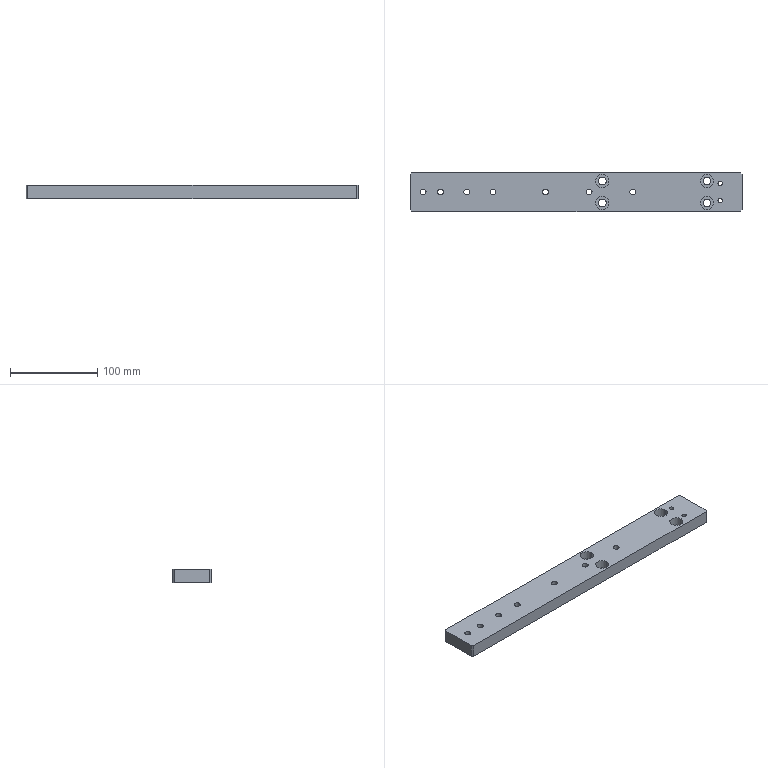Part | SolidWorks | features BaseBody 1 | 1 solid | 48 faces | box 380 x 45 x 15 mm | volume 243637 mm3 | cylinder 34 | plane 14 | commonest cylinder face diameters 6.8 x14 9 x8 15 x8 5 x4
STEP:
#1=CARTESIAN_POINT('',(25.5,12.5,0.));
#2=VERTEX_POINT('',#1);
#3=CARTESIAN_POINT('',(34.5,12.5,0.));
#4=VERTEX_POINT('',#3);
#5=CARTESIAN_POINT('',(30.,12.5,0.));
#6=DIRECTION('',(0.,0.,1.));
#7=DIRECTION('',(1.,0.,0.));
#8=AXIS2_PLACEMENT_3D('',#5,#6,#7);
#9=CIRCLE('',#8,4.5);
#10=EDGE_CURVE('',#2,#4,#9,.T.);
#11=ORIENTED_EDGE('',*,*,#10,.F.);
#12=CARTESIAN_POINT('',(25.5,12.5,5.));
#13=VERTEX_POINT('',#12);
#14=CARTESIAN_POINT('',(25.5,12.5,15.));
#15=DIRECTION('',(0.,0.,1.));
#16=VECTOR('',#15,1000.);
#17=LINE('',#14,#16);
#18=EDGE_CURVE('',#2,#13,#17,.T.);
#19=ORIENTED_EDGE('',*,*,#18,.T.);
#20=CARTESIAN_POINT('',(34.5,12.5,5.));
#21=VERTEX_POINT('',#20);
#22=CARTESIAN_POINT('',(30.,12.5,5.));
#23=DIRECTION('',(0.,0.,-1.));
#24=DIRECTION('',(1.,0.,0.));
#25=AXIS2_PLACEMENT_3D('',#22,#23,#24);
#26=CIRCLE('',#25,4.5);
#27=EDGE_CURVE('',#21,#13,#26,.T.);
#28=ORIENTED_EDGE('',*,*,#27,.F.);
#29=CARTESIAN_POINT('',(34.5,12.5,15.));
#30=DIRECTION('',(0.,0.,1.));
#31=VECTOR('',#30,1000.);
#32=LINE('',#29,#31);
#33=EDGE_CURVE('',#4,#21,#32,.T.);
#34=ORIENTED_EDGE('',*,*,#33,.F.);
#35=EDGE_LOOP('',(#11,#19,#28,#34));
#36=FACE_OUTER_BOUND('',#35,.T.);
#37=CARTESIAN_POINT('',(30.,12.5,15.));
#38=DIRECTION('',(0.,0.,1.));
#39=DIRECTION('',(1.,0.,0.));
#40=AXIS2_PLACEMENT_3D('',#37,#38,#39);
#41=CYLINDRICAL_SURFACE('',#40,4.5);
#42=ADVANCED_FACE('',(#36),#41,.F.);
#43=CARTESIAN_POINT('',(25.5,-12.5,0.));
#44=VERTEX_POINT('',#43);
#45=CARTESIAN_POINT('',(34.5,-12.5,0.));
#46=VERTEX_POINT('',#45);
#47=CARTESIAN_POINT('',(30.,-12.5,0.));
#48=DIRECTION('',(0.,0.,1.));
#49=DIRECTION('',(1.,0.,0.));
#50=AXIS2_PLACEMENT_3D('',#47,#48,#49);
#51=CIRCLE('',#50,4.5);
#52=EDGE_CURVE('',#44,#46,#51,.T.);
#53=ORIENTED_EDGE('',*,*,#52,.F.);
#54=CARTESIAN_POINT('',(25.5,-12.5,5.));
#55=VERTEX_POINT('',#54);
#56=CARTESIAN_POINT('',(25.5,-12.5,15.));
#57=DIRECTION('',(0.,0.,1.));
#58=VECTOR('',#57,1000.);
#59=LINE('',#56,#58);
#60=EDGE_CURVE('',#44,#55,#59,.T.);
#61=ORIENTED_EDGE('',*,*,#60,.T.);
#62=CARTESIAN_POINT('',(34.5,-12.5,5.));
#63=VERTEX_POINT('',#62);
#64=CARTESIAN_POINT('',(30.,-12.5,5.));
#65=DIRECTION('',(0.,0.,-1.));
#66=DIRECTION('',(1.,0.,0.));
#67=AXIS2_PLACEMENT_3D('',#64,#65,#66);
#68=CIRCLE('',#67,4.5);
#69=EDGE_CURVE('',#63,#55,#68,.T.);
#70=ORIENTED_EDGE('',*,*,#69,.F.);
#71=CARTESIAN_POINT('',(34.5,-12.5,15.));
#72=DIRECTION('',(0.,0.,1.));
#73=VECTOR('',#72,1000.);
#74=LINE('',#71,#73);
#75=EDGE_CURVE('',#46,#63,#74,.T.);
#76=ORIENTED_EDGE('',*,*,#75,.F.);
#77=EDGE_LOOP('',(#53,#61,#70,#76));
#78=FACE_OUTER_BOUND('',#77,.T.);
#79=CARTESIAN_POINT('',(30.,-12.5,15.));
#80=DIRECTION('',(0.,0.,1.));
#81=DIRECTION('',(1.,0.,0.));
#82=AXIS2_PLACEMENT_3D('',#79,#80,#81);
#83=CYLINDRICAL_SURFACE('',#82,4.5);
#84=ADVANCED_FACE('',(#78),#83,.F.);
#85=CARTESIAN_POINT('',(145.5,-12.5,0.));
#86=VERTEX_POINT('',#85);
#87=CARTESIAN_POINT('',(154.5,-12.5,0.));
#88=VERTEX_POINT('',#87);
#89=CARTESIAN_POINT('',(150.,-12.5,0.));
#90=DIRECTION('',(0.,0.,1.));
#91=DIRECTION('',(1.,0.,0.));
#92=AXIS2_PLACEMENT_3D('',#89,#90,#91);
#93=CIRCLE('',#92,4.5);
#94=EDGE_CURVE('',#86,#88,#93,.T.);
#95=ORIENTED_EDGE('',*,*,#94,.F.);
#96=CARTESIAN_POINT('',(145.5,-12.5,5.));
#97=VERTEX_POINT('',#96);
#98=CARTESIAN_POINT('',(145.5,-12.5,15.));
#99=DIRECTION('',(0.,0.,1.));
#100=VECTOR('',#99,1000.);
#101=LINE('',#98,#100);
#102=EDGE_CURVE('',#86,#97,#101,.T.);
#103=ORIENTED_EDGE('',*,*,#102,.T.);
#104=CARTESIAN_POINT('',(154.5,-12.5,5.));
#105=VERTEX_POINT('',#104);
#106=CARTESIAN_POINT('',(150.,-12.5,5.));
#107=DIRECTION('',(0.,0.,-1.));
#108=DIRECTION('',(1.,0.,0.));
#109=AXIS2_PLACEMENT_3D('',#106,#107,#108);
#110=CIRCLE('',#109,4.5);
#111=EDGE_CURVE('',#105,#97,#110,.T.);
#112=ORIENTED_EDGE('',*,*,#111,.F.);
#113=CARTESIAN_POINT('',(154.5,-12.5,15.));
#114=DIRECTION('',(0.,0.,1.));
#115=VECTOR('',#114,1000.);
#116=LINE('',#113,#115);
#117=EDGE_CURVE('',#88,#105,#116,.T.);
#118=ORIENTED_EDGE('',*,*,#117,.F.);
#119=EDGE_LOOP('',(#95,#103,#112,#118));
#120=FACE_OUTER_BOUND('',#119,.T.);
#121=CARTESIAN_POINT('',(150.,-12.5,15.));
#122=DIRECTION('',(0.,0.,1.));
#123=DIRECTION('',(1.,0.,0.));
#124=AXIS2_PLACEMENT_3D('',#121,#122,#123);
#125=CYLINDRICAL_SURFACE('',#124,4.5);
#126=ADVANCED_FACE('',(#120),#125,.F.);
#127=CARTESIAN_POINT('',(145.5,12.5,0.));
#128=VERTEX_POINT('',#127);
#129=CARTESIAN_POINT('',(154.5,12.5,0.));
#130=VERTEX_POINT('',#129);
#131=CARTESIAN_POINT('',(150.,12.5,0.));
#132=DIRECTION('',(0.,0.,1.));
#133=DIRECTION('',(1.,0.,0.));
#134=AXIS2_PLACEMENT_3D('',#131,#132,#133);
#135=CIRCLE('',#134,4.5);
#136=EDGE_CURVE('',#128,#130,#135,.T.);
#137=ORIENTED_EDGE('',*,*,#136,.F.);
#138=CARTESIAN_POINT('',(145.5,12.5,5.));
#139=VERTEX_POINT('',#138);
#140=CARTESIAN_POINT('',(145.5,12.5,15.));
#141=DIRECTION('',(0.,0.,1.));
#142=VECTOR('',#141,1000.);
#143=LINE('',#140,#142);
#144=EDGE_CURVE('',#128,#139,#143,.T.);
#145=ORIENTED_EDGE('',*,*,#144,.T.);
#146=CARTESIAN_POINT('',(154.5,12.5,5.));
#147=VERTEX_POINT('',#146);
#148=CARTESIAN_POINT('',(150.,12.5,5.));
#149=DIRECTION('',(0.,0.,-1.));
#150=DIRECTION('',(1.,0.,0.));
#151=AXIS2_PLACEMENT_3D('',#148,#149,#150);
#152=CIRCLE('',#151,4.5);
#153=EDGE_CURVE('',#147,#139,#152,.T.);
#154=ORIENTED_EDGE('',*,*,#153,.F.);
#155=CARTESIAN_POINT('',(154.5,12.5,15.));
#156=DIRECTION('',(0.,0.,1.));
#157=VECTOR('',#156,1000.);
#158=LINE('',#155,#157);
#159=EDGE_CURVE('',#130,#147,#158,.T.);
#160=ORIENTED_EDGE('',*,*,#159,.F.);
#161=EDGE_LOOP('',(#137,#145,#154,#160));
#162=FACE_OUTER_BOUND('',#161,.T.);
#163=CARTESIAN_POINT('',(150.,12.5,15.));
#164=DIRECTION('',(0.,0.,1.));
#165=DIRECTION('',(1.,0.,0.));
#166=AXIS2_PLACEMENT_3D('',#163,#164,#165);
#167=CYLINDRICAL_SURFACE('',#166,4.5);
#168=ADVANCED_FACE('',(#162),#167,.F.);
#169=CARTESIAN_POINT('',(-178.4,0.,0.));
#170=VERTEX_POINT('',#169);
#171=CARTESIAN_POINT('',(-171.6,0.,0.));
#172=VERTEX_POINT('',#171);
#173=CARTESIAN_POINT('',(-175.,0.,0.));
#174=DIRECTION('',(0.,0.,1.));
#175=DIRECTION('',(1.,0.,0.));
#176=AXIS2_PLACEMENT_3D('',#173,#174,#175);
#177=CIRCLE('',#176,3.4);
#178=EDGE_CURVE('',#170,#172,#177,.T.);
#179=ORIENTED_EDGE('',*,*,#178,.F.);
#180=CARTESIAN_POINT('',(-178.4,0.,15.));
#181=VERTEX_POINT('',#180);
#182=CARTESIAN_POINT('',(-178.4,0.,15.));
#183=DIRECTION('',(0.,0.,1.));
#184=VECTOR('',#183,1000.);
#185=LINE('',#182,#184);
#186=EDGE_CURVE('',#170,#181,#185,.T.);
#187=ORIENTED_EDGE('',*,*,#186,.T.);
#188=CARTESIAN_POINT('',(-171.6,0.,15.));
#189=VERTEX_POINT('',#188);
#190=CARTESIAN_POINT('',(-175.,0.,15.));
#191=DIRECTION('',(0.,0.,-1.));
#192=DIRECTION('',(1.,0.,0.));
#193=AXIS2_PLACEMENT_3D('',#190,#191,#192);
#194=CIRCLE('',#193,3.4);
#195=EDGE_CURVE('',#189,#181,#194,.T.);
#196=ORIENTED_EDGE('',*,*,#195,.F.);
#197=CARTESIAN_POINT('',(-171.6,0.,15.));
#198=DIRECTION('',(0.,0.,1.));
#199=VECTOR('',#198,1000.);
#200=LINE('',#197,#199);
#201=EDGE_CURVE('',#172,#189,#200,.T.);
#202=ORIENTED_EDGE('',*,*,#201,.F.);
#203=EDGE_LOOP('',(#179,#187,#196,#202));
#204=FACE_OUTER_BOUND('',#203,.T.);
#205=CARTESIAN_POINT('',(-175.,0.,15.));
#206=DIRECTION('',(0.,0.,1.));
#207=DIRECTION('',(1.,0.,0.));
#208=AXIS2_PLACEMENT_3D('',#205,#206,#207);
#209=CYLINDRICAL_SURFACE('',#208,3.4);
#210=ADVANCED_FACE('',(#204),#209,.F.);
#211=CARTESIAN_POINT('',(61.6,0.,0.));
#212=VERTEX_POINT('',#211);
#213=CARTESIAN_POINT('',(68.4,0.,0.));
#214=VERTEX_POINT('',#213);
#215=CARTESIAN_POINT('',(65.,0.,0.));
#216=DIRECTION('',(0.,0.,1.));
#217=DIRECTION('',(1.,0.,0.));
#218=AXIS2_PLACEMENT_3D('',#215,#216,#217);
#219=CIRCLE('',#218,3.4);
#220=EDGE_CURVE('',#212,#214,#219,.T.);
#221=ORIENTED_EDGE('',*,*,#220,.F.);
#222=CARTESIAN_POINT('',(61.6,0.,15.));
#223=VERTEX_POINT('',#222);
#224=CARTESIAN_POINT('',(61.6,0.,15.));
#225=DIRECTION('',(0.,0.,1.));
#226=VECTOR('',#225,1000.);
#227=LINE('',#224,#226);
#228=EDGE_CURVE('',#212,#223,#227,.T.);
#229=ORIENTED_EDGE('',*,*,#228,.T.);
#230=CARTESIAN_POINT('',(68.4,0.,15.));
#231=VERTEX_POINT('',#230);
#232=CARTESIAN_POINT('',(65.,0.,15.));
#233=DIRECTION('',(0.,0.,-1.));
#234=DIRECTION('',(1.,0.,0.));
#235=AXIS2_PLACEMENT_3D('',#232,#233,#234);
#236=CIRCLE('',#235,3.4);
#237=EDGE_CURVE('',#231,#223,#236,.T.);
#238=ORIENTED_EDGE('',*,*,#237,.F.);
#239=CARTESIAN_POINT('',(68.4,0.,15.));
#240=DIRECTION('',(0.,0.,1.));
#241=VECTOR('',#240,1000.);
#242=LINE('',#239,#241);
#243=EDGE_CURVE('',#214,#231,#242,.T.);
#244=ORIENTED_EDGE('',*,*,#243,.F.);
#245=EDGE_LOOP('',(#221,#229,#238,#244));
#246=FACE_OUTER_BOUND('',#245,.T.);
#247=CARTESIAN_POINT('',(65.,0.,15.));
#248=DIRECTION('',(0.,0.,1.));
#249=DIRECTION('',(1.,0.,0.));
#250=AXIS2_PLACEMENT_3D('',#247,#248,#249);
#251=CYLINDRICAL_SURFACE('',#250,3.4);
#252=ADVANCED_FACE('',(#246),#251,.F.);
#253=CARTESIAN_POINT('',(11.6,0.,0.));
#254=VERTEX_POINT('',#253);
#255=CARTESIAN_POINT('',(18.4,0.,0.));
#256=VERTEX_POINT('',#255);
#257=CARTESIAN_POINT('',(15.,0.,0.));
#258=DIRECTION('',(0.,0.,1.));
#259=DIRECTION('',(1.,0.,0.));
#260=AXIS2_PLACEMENT_3D('',#257,#258,#259);
#261=CIRCLE('',#260,3.4);
#262=EDGE_CURVE('',#254,#256,#261,.T.);
#263=ORIENTED_EDGE('',*,*,#262,.F.);
#264=CARTESIAN_POINT('',(11.6,0.,15.));
#265=VERTEX_POINT('',#264);
#266=CARTESIAN_POINT('',(11.6,0.,15.));
#267=DIRECTION('',(0.,0.,1.));
#268=VECTOR('',#267,1000.);
#269=LINE('',#266,#268);
#270=EDGE_CURVE('',#254,#265,#269,.T.);
#271=ORIENTED_EDGE('',*,*,#270,.T.);
#272=CARTESIAN_POINT('',(18.4,0.,15.));
#273=VERTEX_POINT('',#272);
#274=CARTESIAN_POINT('',(15.,0.,15.));
#275=DIRECTION('',(0.,0.,-1.));
#276=DIRECTION('',(1.,0.,0.));
#277=AXIS2_PLACEMENT_3D('',#274,#275,#276);
#278=CIRCLE('',#277,3.4);
#279=EDGE_CURVE('',#273,#265,#278,.T.);
#280=ORIENTED_EDGE('',*,*,#279,.F.);
#281=CARTESIAN_POINT('',(18.4,0.,15.));
#282=DIRECTION('',(0.,0.,1.));
#283=VECTOR('',#282,1000.);
#284=LINE('',#281,#283);
#285=EDGE_CURVE('',#256,#273,#284,.T.);
#286=ORIENTED_EDGE('',*,*,#285,.F.);
#287=EDGE_LOOP('',(#263,#271,#280,#286));
#288=FACE_OUTER_BOUND('',#287,.T.);
#289=CARTESIAN_POINT('',(15.,0.,15.));
#290=DIRECTION('',(0.,0.,1.));
#291=DIRECTION('',(1.,0.,0.));
#292=AXIS2_PLACEMENT_3D('',#289,#290,#291);
#293=CYLINDRICAL_SURFACE('',#292,3.4);
#294=ADVANCED_FACE('',(#288),#293,.F.);
#295=CARTESIAN_POINT('',(-38.4,0.,0.));
#296=VERTEX_POINT('',#295);
#297=CARTESIAN_POINT('',(-31.6,0.,0.));
#298=VERTEX_POINT('',#297);
#299=CARTESIAN_POINT('',(-35.,0.,0.));
#300=DIRECTION('',(0.,0.,1.));
#301=DIRECTION('',(1.,0.,0.));
#302=AXIS2_PLACEMENT_3D('',#299,#300,#301);
#303=CIRCLE('',#302,3.4);
#304=EDGE_CURVE('',#296,#298,#303,.T.);
#305=ORIENTED_EDGE('',*,*,#304,.F.);
#306=CARTESIAN_POINT('',(-38.4,0.,15.));
#307=VERTEX_POINT('',#306);
#308=CARTESIAN_POINT('',(-38.4,0.,15.));
#309=DIRECTION('',(0.,0.,1.));
#310=VECTOR('',#309,1000.);
#311=LINE('',#308,#310);
#312=EDGE_CURVE('',#296,#307,#311,.T.);
#313=ORIENTED_EDGE('',*,*,#312,.T.);
#314=CARTESIAN_POINT('',(-31.6,0.,15.));
#315=VERTEX_POINT('',#314);
#316=CARTESIAN_POINT('',(-35.,0.,15.));
#317=DIRECTION('',(0.,0.,-1.));
#318=DIRECTION('',(1.,0.,0.));
#319=AXIS2_PLACEMENT_3D('',#316,#317,#318);
#320=CIRCLE('',#319,3.4);
#321=EDGE_CURVE('',#315,#307,#320,.T.);
#322=ORIENTED_EDGE('',*,*,#321,.F.);
#323=CARTESIAN_POINT('',(-31.6,0.,15.));
#324=DIRECTION('',(0.,0.,1.));
#325=VECTOR('',#324,1000.);
#326=LINE('',#323,#325);
#327=EDGE_CURVE('',#298,#315,#326,.T.);
#328=ORIENTED_EDGE('',*,*,#327,.F.);
#329=EDGE_LOOP('',(#305,#313,#322,#328));
#330=FACE_OUTER_BOUND('',#329,.T.);
#331=CARTESIAN_POINT('',(-35.,0.,15.));
#332=DIRECTION('',(0.,0.,1.));
#333=DIRECTION('',(1.,0.,0.));
#334=AXIS2_PLACEMENT_3D('',#331,#332,#333);
#335=CYLINDRICAL_SURFACE('',#334,3.4);
#336=ADVANCED_FACE('',(#330),#335,.F.);
#337=CARTESIAN_POINT('',(-98.4,0.,0.));
#338=VERTEX_POINT('',#337);
#339=CARTESIAN_POINT('',(-91.6,0.,0.));
#340=VERTEX_POINT('',#339);
#341=CARTESIAN_POINT('',(-95.,0.,0.));
#342=DIRECTION('',(0.,0.,1.));
#343=DIRECTION('',(1.,0.,0.));
#344=AXIS2_PLACEMENT_3D('',#341,#342,#343);
#345=CIRCLE('',#344,3.4);
#346=EDGE_CURVE('',#338,#340,#345,.T.);
#347=ORIENTED_EDGE('',*,*,#346,.F.);
#348=CARTESIAN_POINT('',(-98.4,0.,15.));
#349=VERTEX_POINT('',#348);
#350=CARTESIAN_POINT('',(-98.4,0.,15.));
#351=DIRECTION('',(0.,0.,1.));
#352=VECTOR('',#351,1000.);
#353=LINE('',#350,#352);
#354=EDGE_CURVE('',#338,#349,#353,.T.);
#355=ORIENTED_EDGE('',*,*,#354,.T.);
#356=CARTESIAN_POINT('',(-91.6,0.,15.));
#357=VERTEX_POINT('',#356);
#358=CARTESIAN_POINT('',(-95.,0.,15.));
#359=DIRECTION('',(0.,0.,-1.));
#360=DIRECTION('',(1.,0.,0.));
#361=AXIS2_PLACEMENT_3D('',#358,#359,#360);
#362=CIRCLE('',#361,3.4);
#363=EDGE_CURVE('',#357,#349,#362,.T.);
#364=ORIENTED_EDGE('',*,*,#363,.F.);
#365=CARTESIAN_POINT('',(-91.6,0.,15.));
#366=DIRECTION('',(0.,0.,1.));
#367=VECTOR('',#366,1000.);
#368=LINE('',#365,#367);
#369=EDGE_CURVE('',#340,#357,#368,.T.);
#370=ORIENTED_EDGE('',*,*,#369,.F.);
#371=EDGE_LOOP('',(#347,#355,#364,#370));
#372=FACE_OUTER_BOUND('',#371,.T.);
#373=CARTESIAN_POINT('',(-95.,0.,15.));
#374=DIRECTION('',(0.,0.,1.));
#375=DIRECTION('',(1.,0.,0.));
#376=AXIS2_PLACEMENT_3D('',#373,#374,#375);
#377=CYLINDRICAL_SURFACE('',#376,3.4);
#378=ADVANCED_FACE('',(#372),#377,.F.);
#379=CARTESIAN_POINT('',(-128.4,0.,0.));
#380=VERTEX_POINT('',#379);
#381=CARTESIAN_POINT('',(-121.6,0.,0.));
#382=VERTEX_POINT('',#381);
#383=CARTESIAN_POINT('',(-125.,0.,0.));
#384=DIRECTION('',(0.,0.,1.));
#385=DIRECTION('',(1.,0.,0.));
#386=AXIS2_PLACEMENT_3D('',#383,#384,#385);
#387=CIRCLE('',#386,3.4);
#388=EDGE_CURVE('',#380,#382,#387,.T.);
#389=ORIENTED_EDGE('',*,*,#388,.F.);
#390=CARTESIAN_POINT('',(-128.4,0.,15.));
#391=VERTEX_POINT('',#390);
#392=CARTESIAN_POINT('',(-128.4,0.,15.));
#393=DIRECTION('',(0.,0.,1.));
#394=VECTOR('',#393,1000.);
#395=LINE('',#392,#394);
#396=EDGE_CURVE('',#380,#391,#395,.T.);
#397=ORIENTED_EDGE('',*,*,#396,.T.);
#398=CARTESIAN_POINT('',(-121.6,0.,15.));
#399=VERTEX_POINT('',#398);
#400=CARTESIAN_POINT('',(-125.,0.,15.));
#401=DIRECTION('',(0.,0.,-1.));
#402=DIRECTION('',(1.,0.,0.));
#403=AXIS2_PLACEMENT_3D('',#400,#401,#402);
#404=CIRCLE('',#403,3.4);
#405=EDGE_CURVE('',#399,#391,#404,.T.);
#406=ORIENTED_EDGE('',*,*,#405,.F.);
#407=CARTESIAN_POINT('',(-121.6,0.,15.));
#408=DIRECTION('',(0.,0.,1.));
#409=VECTOR('',#408,1000.);
#410=LINE('',#407,#409);
#411=EDGE_CURVE('',#382,#399,#410,.T.);
#412=ORIENTED_EDGE('',*,*,#411,.F.);
#413=EDGE_LOOP('',(#389,#397,#406,#412));
#414=FACE_OUTER_BOUND('',#413,.T.);
#415=CARTESIAN_POINT('',(-125.,0.,15.));
#416=DIRECTION('',(0.,0.,1.));
#417=DIRECTION('',(1.,0.,0.));
#418=AXIS2_PLACEMENT_3D('',#415,#416,#417);
#419=CYLINDRICAL_SURFACE('',#418,3.4);
#420=ADVANCED_FACE('',(#414),#419,.F.);
#421=CARTESIAN_POINT('',(-158.4,0.,0.));
#422=VERTEX_POINT('',#421);
#423=CARTESIAN_POINT('',(-151.6,0.,0.));
#424=VERTEX_POINT('',#423);
#425=CARTESIAN_POINT('',(-155.,0.,0.));
#426=DIRECTION('',(0.,0.,1.));
#427=DIRECTION('',(1.,0.,0.));
#428=AXIS2_PLACEMENT_3D('',#425,#426,#427);
#429=CIRCLE('',#428,3.4);
#430=EDGE_CURVE('',#422,#424,#429,.T.);
#431=ORIENTED_EDGE('',*,*,#430,.F.);
#432=CARTESIAN_POINT('',(-158.4,0.,15.));
#433=VERTEX_POINT('',#432);
#434=CARTESIAN_POINT('',(-158.4,0.,15.));
#435=DIRECTION('',(0.,0.,1.));
#436=VECTOR('',#435,1000.);
#437=LINE('',#434,#436);
#438=EDGE_CURVE('',#422,#433,#437,.T.);
#439=ORIENTED_EDGE('',*,*,#438,.T.);
#440=CARTESIAN_POINT('',(-151.6,0.,15.));
#441=VERTEX_POINT('',#440);
#442=CARTESIAN_POINT('',(-155.,0.,15.));
#443=DIRECTION('',(0.,0.,-1.));
#444=DIRECTION('',(1.,0.,0.));
#445=AXIS2_PLACEMENT_3D('',#442,#443,#444);
#446=CIRCLE('',#445,3.4);
#447=EDGE_CURVE('',#441,#433,#446,.T.);
#448=ORIENTED_EDGE('',*,*,#447,.F.);
#449=CARTESIAN_POINT('',(-151.6,0.,15.));
#450=DIRECTION('',(0.,0.,1.));
#451=VECTOR('',#450,1000.);
#452=LINE('',#449,#451);
#453=EDGE_CURVE('',#424,#441,#452,.T.);
#454=ORIENTED_EDGE('',*,*,#453,.F.);
#455=EDGE_LOOP('',(#431,#439,#448,#454));
#456=FACE_OUTER_BOUND('',#455,.T.);
#457=CARTESIAN_POINT('',(-155.,0.,15.));
#458=DIRECTION('',(0.,0.,1.));
#459=DIRECTION('',(1.,0.,0.));
#460=AXIS2_PLACEMENT_3D('',#457,#458,#459);
#461=CYLINDRICAL_SURFACE('',#460,3.4);
#462=ADVANCED_FACE('',(#456),#461,.F.);
#463=CARTESIAN_POINT('',(162.5,-10.,0.));
#464=VERTEX_POINT('',#463);
#465=CARTESIAN_POINT('',(167.5,-10.,0.));
#466=VERTEX_POINT('',#465);
#467=CARTESIAN_POINT('',(165.,-10.,0.));
#468=DIRECTION('',(0.,0.,1.));
#469=DIRECTION('',(1.,0.,0.));
#470=AXIS2_PLACEMENT_3D('',#467,#468,#469);
#471=CIRCLE('',#470,2.5);
#472=EDGE_CURVE('',#464,#466,#471,.T.);
#473=ORIENTED_EDGE('',*,*,#472,.F.);
#474=CARTESIAN_POINT('',(162.5,-10.,15.));
#475=VERTEX_POINT('',#474);
#476=CARTESIAN_POINT('',(162.5,-10.,15.));
#477=DIRECTION('',(0.,0.,1.));
#478=VECTOR('',#477,1000.);
#479=LINE('',#476,#478);
#480=EDGE_CURVE('',#464,#475,#479,.T.);
#481=ORIENTED_EDGE('',*,*,#480,.T.);
#482=CARTESIAN_POINT('',(167.5,-10.,15.));
#483=VERTEX_POINT('',#482);
#484=CARTESIAN_POINT('',(165.,-10.,15.));
#485=DIRECTION('',(0.,0.,-1.));
#486=DIRECTION('',(1.,0.,0.));
#487=AXIS2_PLACEMENT_3D('',#484,#485,#486);
#488=CIRCLE('',#487,2.5);
#489=EDGE_CURVE('',#483,#475,#488,.T.);
#490=ORIENTED_EDGE('',*,*,#489,.F.);
#491=CARTESIAN_POINT('',(167.5,-10.,15.));
#492=DIRECTION('',(0.,0.,1.));
#493=VECTOR('',#492,1000.);
#494=LINE('',#491,#493);
#495=EDGE_CURVE('',#466,#483,#494,.T.);
#496=ORIENTED_EDGE('',*,*,#495,.F.);
#497=EDGE_LOOP('',(#473,#481,#490,#496));
#498=FACE_OUTER_BOUND('',#497,.T.);
#499=CARTESIAN_POINT('',(165.,-10.,15.));
#500=DIRECTION('',(0.,0.,1.));
#501=DIRECTION('',(1.,0.,0.));
#502=AXIS2_PLACEMENT_3D('',#499,#500,#501);
#503=CYLINDRICAL_SURFACE('',#502,2.5);
#504=ADVANCED_FACE('',(#498),#503,.F.);
#505=CARTESIAN_POINT('',(162.5,10.,0.));
#506=VERTEX_POINT('',#505);
#507=CARTESIAN_POINT('',(167.5,10.,0.));
#508=VERTEX_POINT('',#507);
#509=CARTESIAN_POINT('',(165.,10.,0.));
#510=DIRECTION('',(0.,0.,1.));
#511=DIRECTION('',(1.,0.,0.));
#512=AXIS2_PLACEMENT_3D('',#509,#510,#511);
#513=CIRCLE('',#512,2.5);
#514=EDGE_CURVE('',#506,#508,#513,.T.);
#515=ORIENTED_EDGE('',*,*,#514,.F.);
#516=CARTESIAN_POINT('',(162.5,10.,15.));
#517=VERTEX_POINT('',#516);
#518=CARTESIAN_POINT('',(162.5,10.,15.));
#519=DIRECTION('',(0.,0.,1.));
#520=VECTOR('',#519,1000.);
#521=LINE('',#518,#520);
#522=EDGE_CURVE('',#506,#517,#521,.T.);
#523=ORIENTED_EDGE('',*,*,#522,.T.);
#524=CARTESIAN_POINT('',(167.5,10.,15.));
#525=VERTEX_POINT('',#524);
#526=CARTESIAN_POINT('',(165.,10.,15.));
#527=DIRECTION('',(0.,0.,-1.));
#528=DIRECTION('',(1.,0.,0.));
#529=AXIS2_PLACEMENT_3D('',#526,#527,#528);
#530=CIRCLE('',#529,2.5);
#531=EDGE_CURVE('',#525,#517,#530,.T.);
#532=ORIENTED_EDGE('',*,*,#531,.F.);
#533=CARTESIAN_POINT('',(167.5,10.,15.));
#534=DIRECTION('',(0.,0.,1.));
#535=VECTOR('',#534,1000.);
#536=LINE('',#533,#535);
#537=EDGE_CURVE('',#508,#525,#536,.T.);
#538=ORIENTED_EDGE('',*,*,#537,.F.);
#539=EDGE_LOOP('',(#515,#523,#532,#538));
#540=FACE_OUTER_BOUND('',#539,.T.);
#541=CARTESIAN_POINT('',(165.,10.,15.));
#542=DIRECTION('',(0.,0.,1.));
#543=DIRECTION('',(1.,0.,0.));
#544=AXIS2_PLACEMENT_3D('',#541,#542,#543);
#545=CYLINDRICAL_SURFACE('',#544,2.5);
#546=ADVANCED_FACE('',(#540),#545,.F.);
#547=CARTESIAN_POINT('',(37.5,12.5,5.));
#548=VERTEX_POINT('',#547);
#549=CARTESIAN_POINT('',(22.5,12.5,5.));
#550=VERTEX_POINT('',#549);
#551=CARTESIAN_POINT('',(30.,12.5,5.));
#552=DIRECTION('',(0.,0.,-1.));
#553=DIRECTION('',(1.,0.,0.));
#554=AXIS2_PLACEMENT_3D('',#551,#552,#553);
#555=CIRCLE('',#554,7.5);
#556=EDGE_CURVE('',#548,#550,#555,.T.);
#557=ORIENTED_EDGE('',*,*,#556,.T.);
#558=CARTESIAN_POINT('',(22.5,12.5,15.));
#559=VERTEX_POINT('',#558);
#560=CARTESIAN_POINT('',(22.5,12.5,15.));
#561=DIRECTION('',(0.,0.,1.));
#562=VECTOR('',#561,1000.);
#563=LINE('',#560,#562);
#564=EDGE_CURVE('',#550,#559,#563,.T.);
#565=ORIENTED_EDGE('',*,*,#564,.T.);
#566=CARTESIAN_POINT('',(37.5,12.5,15.));
#567=VERTEX_POINT('',#566);
#568=CARTESIAN_POINT('',(30.,12.5,15.));
#569=DIRECTION('',(0.,0.,1.));
#570=DIRECTION('',(1.,0.,0.));
#571=AXIS2_PLACEMENT_3D('',#568,#569,#570);
#572=CIRCLE('',#571,7.5);
#573=EDGE_CURVE('',#559,#567,#572,.T.);
#574=ORIENTED_EDGE('',*,*,#573,.T.);
#575=CARTESIAN_POINT('',(37.5,12.5,15.));
#576=DIRECTION('',(0.,0.,1.));
#577=VECTOR('',#576,1000.);
#578=LINE('',#575,#577);
#579=EDGE_CURVE('',#548,#567,#578,.T.);
#580=ORIENTED_EDGE('',*,*,#579,.F.);
#581=EDGE_LOOP('',(#557,#565,#574,#580));
#582=FACE_OUTER_BOUND('',#581,.T.);
#583=CARTESIAN_POINT('',(30.,12.5,15.));
#584=DIRECTION('',(0.,0.,1.));
#585=DIRECTION('',(1.,0.,0.));
#586=AXIS2_PLACEMENT_3D('',#583,#584,#585);
#587=CYLINDRICAL_SURFACE('',#586,7.5);
#588=ADVANCED_FACE('',(#582),#587,.F.);
#589=CARTESIAN_POINT('',(37.5,-12.5,5.));
#590=VERTEX_POINT('',#589);
#591=CARTESIAN_POINT('',(22.5,-12.5,5.));
#592=VERTEX_POINT('',#591);
#593=CARTESIAN_POINT('',(30.,-12.5,5.));
#594=DIRECTION('',(0.,0.,-1.));
#595=DIRECTION('',(1.,0.,0.));
#596=AXIS2_PLACEMENT_3D('',#593,#594,#595);
#597=CIRCLE('',#596,7.5);
#598=EDGE_CURVE('',#590,#592,#597,.T.);
#599=ORIENTED_EDGE('',*,*,#598,.T.);
#600=CARTESIAN_POINT('',(22.5,-12.5,15.));
#601=VERTEX_POINT('',#600);
#602=CARTESIAN_POINT('',(22.5,-12.5,15.));
#603=DIRECTION('',(0.,0.,1.));
#604=VECTOR('',#603,1000.);
#605=LINE('',#602,#604);
#606=EDGE_CURVE('',#592,#601,#605,.T.);
#607=ORIENTED_EDGE('',*,*,#606,.T.);
#608=CARTESIAN_POINT('',(37.5,-12.5,15.));
#609=VERTEX_POINT('',#608);
#610=CARTESIAN_POINT('',(30.,-12.5,15.));
#611=DIRECTION('',(0.,0.,1.));
#612=DIRECTION('',(1.,0.,0.));
#613=AXIS2_PLACEMENT_3D('',#610,#611,#612);
#614=CIRCLE('',#613,7.5);
#615=EDGE_CURVE('',#601,#609,#614,.T.);
#616=ORIENTED_EDGE('',*,*,#615,.T.);
#617=CARTESIAN_POINT('',(37.5,-12.5,15.));
#618=DIRECTION('',(0.,0.,1.));
#619=VECTOR('',#618,1000.);
#620=LINE('',#617,#619);
#621=EDGE_CURVE('',#590,#609,#620,.T.);
#622=ORIENTED_EDGE('',*,*,#621,.F.);
#623=EDGE_LOOP('',(#599,#607,#616,#622));
#624=FACE_OUTER_BOUND('',#623,.T.);
#625=CARTESIAN_POINT('',(30.,-12.5,15.));
#626=DIRECTION('',(0.,0.,1.));
#627=DIRECTION('',(1.,0.,0.));
#628=AXIS2_PLACEMENT_3D('',#625,#626,#627);
#629=CYLINDRICAL_SURFACE('',#628,7.5);
#630=ADVANCED_FACE('',(#624),#629,.F.);
#631=CARTESIAN_POINT('',(157.5,-12.5,5.));
#632=VERTEX_POINT('',#631);
#633=CARTESIAN_POINT('',(142.5,-12.5,5.));
#634=VERTEX_POINT('',#633);
#635=CARTESIAN_POINT('',(150.,-12.5,5.));
#636=DIRECTION('',(0.,0.,-1.));
#637=DIRECTION('',(1.,0.,0.));
#638=AXIS2_PLACEMENT_3D('',#635,#636,#637);
#639=CIRCLE('',#638,7.5);
#640=EDGE_CURVE('',#632,#634,#639,.T.);
#641=ORIENTED_EDGE('',*,*,#640,.T.);
#642=CARTESIAN_POINT('',(142.5,-12.5,15.));
#643=VERTEX_POINT('',#642);
#644=CARTESIAN_POINT('',(142.5,-12.5,15.));
#645=DIRECTION('',(0.,0.,1.));
#646=VECTOR('',#645,1000.);
#647=LINE('',#644,#646);
#648=EDGE_CURVE('',#634,#643,#647,.T.);
#649=ORIENTED_EDGE('',*,*,#648,.T.);
#650=CARTESIAN_POINT('',(157.5,-12.5,15.));
#651=VERTEX_POINT('',#650);
#652=CARTESIAN_POINT('',(150.,-12.5,15.));
#653=DIRECTION('',(0.,0.,1.));
#654=DIRECTION('',(1.,0.,0.));
#655=AXIS2_PLACEMENT_3D('',#652,#653,#654);
#656=CIRCLE('',#655,7.5);
#657=EDGE_CURVE('',#643,#651,#656,.T.);
#658=ORIENTED_EDGE('',*,*,#657,.T.);
#659=CARTESIAN_POINT('',(157.5,-12.5,15.));
#660=DIRECTION('',(0.,0.,1.));
#661=VECTOR('',#660,1000.);
#662=LINE('',#659,#661);
#663=EDGE_CURVE('',#632,#651,#662,.T.);
#664=ORIENTED_EDGE('',*,*,#663,.F.);
#665=EDGE_LOOP('',(#641,#649,#658,#664));
#666=FACE_OUTER_BOUND('',#665,.T.);
#667=CARTESIAN_POINT('',(150.,-12.5,15.));
#668=DIRECTION('',(0.,0.,1.));
#669=DIRECTION('',(1.,0.,0.));
#670=AXIS2_PLACEMENT_3D('',#667,#668,#669);
#671=CYLINDRICAL_SURFACE('',#670,7.5);
#672=ADVANCED_FACE('',(#666),#671,.F.);
#673=CARTESIAN_POINT('',(157.5,12.5,5.));
#674=VERTEX_POINT('',#673);
#675=CARTESIAN_POINT('',(142.5,12.5,5.));
#676=VERTEX_POINT('',#675);
#677=CARTESIAN_POINT('',(150.,12.5,5.));
#678=DIRECTION('',(0.,0.,-1.));
#679=DIRECTION('',(1.,0.,0.));
#680=AXIS2_PLACEMENT_3D('',#677,#678,#679);
#681=CIRCLE('',#680,7.5);
#682=EDGE_CURVE('',#674,#676,#681,.T.);
#683=ORIENTED_EDGE('',*,*,#682,.T.);
#684=CARTESIAN_POINT('',(142.5,12.5,15.));
#685=VERTEX_POINT('',#684);
#686=CARTESIAN_POINT('',(142.5,12.5,15.));
#687=DIRECTION('',(0.,0.,1.));
#688=VECTOR('',#687,1000.);
#689=LINE('',#686,#688);
#690=EDGE_CURVE('',#676,#685,#689,.T.);
#691=ORIENTED_EDGE('',*,*,#690,.T.);
#692=CARTESIAN_POINT('',(157.5,12.5,15.));
#693=VERTEX_POINT('',#692);
#694=CARTESIAN_POINT('',(150.,12.5,15.));
#695=DIRECTION('',(0.,0.,1.));
#696=DIRECTION('',(1.,0.,0.));
#697=AXIS2_PLACEMENT_3D('',#694,#695,#696);
#698=CIRCLE('',#697,7.5);
#699=EDGE_CURVE('',#685,#693,#698,.T.);
#700=ORIENTED_EDGE('',*,*,#699,.T.);
#701=CARTESIAN_POINT('',(157.5,12.5,15.));
#702=DIRECTION('',(0.,0.,1.));
#703=VECTOR('',#702,1000.);
#704=LINE('',#701,#703);
#705=EDGE_CURVE('',#674,#693,#704,.T.);
#706=ORIENTED_EDGE('',*,*,#705,.F.);
#707=EDGE_LOOP('',(#683,#691,#700,#706));
#708=FACE_OUTER_BOUND('',#707,.T.);
#709=CARTESIAN_POINT('',(150.,12.5,15.));
#710=DIRECTION('',(0.,0.,1.));
#711=DIRECTION('',(1.,0.,0.));
#712=AXIS2_PLACEMENT_3D('',#709,#710,#711);
#713=CYLINDRICAL_SURFACE('',#712,7.5);
#714=ADVANCED_FACE('',(#708),#713,.F.);
#715=CARTESIAN_POINT('',(188.,-22.5,0.));
#716=VERTEX_POINT('',#715);
#717=CARTESIAN_POINT('',(-188.,-22.5,0.));
#718=VERTEX_POINT('',#717);
#719=CARTESIAN_POINT('',(0.,-22.5,0.));
#720=DIRECTION('',(-1.,0.,0.));
#721=VECTOR('',#720,1000.);
#722=LINE('',#719,#721);
#723=EDGE_CURVE('',#716,#718,#722,.T.);
#724=ORIENTED_EDGE('',*,*,#723,.T.);
#725=CARTESIAN_POINT('',(-190.,-20.5,0.));
#726=VERTEX_POINT('',#725);
#727=CARTESIAN_POINT('',(-188.,-22.5,0.));
#728=DIRECTION('',(-0.7071,0.7071,0.));
#729=VECTOR('',#728,1000.);
#730=LINE('',#727,#729);
#731=EDGE_CURVE('',#718,#726,#730,.T.);
#732=ORIENTED_EDGE('',*,*,#731,.T.);
#733=CARTESIAN_POINT('',(-190.,20.5,0.));
#734=VERTEX_POINT('',#733);
#735=CARTESIAN_POINT('',(-190.,0.,0.));
#736=DIRECTION('',(0.,1.,0.));
#737=VECTOR('',#736,1000.);
#738=LINE('',#735,#737);
#739=EDGE_CURVE('',#726,#734,#738,.T.);
#740=ORIENTED_EDGE('',*,*,#739,.T.);
#741=CARTESIAN_POINT('',(-188.,22.5,0.));
#742=VERTEX_POINT('',#741);
#743=CARTESIAN_POINT('',(-190.,20.5,0.));
#744=DIRECTION('',(0.7071,0.7071,0.));
#745=VECTOR('',#744,1000.);
#746=LINE('',#743,#745);
#747=EDGE_CURVE('',#734,#742,#746,.T.);
#748=ORIENTED_EDGE('',*,*,#747,.T.);
#749=CARTESIAN_POINT('',(188.,22.5,0.));
#750=VERTEX_POINT('',#749);
#751=CARTESIAN_POINT('',(0.,22.5,0.));
#752=DIRECTION('',(1.,0.,0.));
#753=VECTOR('',#752,1000.);
#754=LINE('',#751,#753);
#755=EDGE_CURVE('',#742,#750,#754,.T.);
#756=ORIENTED_EDGE('',*,*,#755,.T.);
#757=CARTESIAN_POINT('',(190.,20.5,0.));
#758=VERTEX_POINT('',#757);
#759=CARTESIAN_POINT('',(188.,22.5,0.));
#760=DIRECTION('',(0.7071,-0.7071,0.));
#761=VECTOR('',#760,1000.);
#762=LINE('',#759,#761);
#763=EDGE_CURVE('',#750,#758,#762,.T.);
#764=ORIENTED_EDGE('',*,*,#763,.T.);
#765=CARTESIAN_POINT('',(190.,-20.5,0.));
#766=VERTEX_POINT('',#765);
#767=CARTESIAN_POINT('',(190.,0.,0.));
#768=DIRECTION('',(0.,-1.,0.));
#769=VECTOR('',#768,1000.);
#770=LINE('',#767,#769);
#771=EDGE_CURVE('',#758,#766,#770,.T.);
#772=ORIENTED_EDGE('',*,*,#771,.T.);
#773=CARTESIAN_POINT('',(190.,-20.5,0.));
#774=DIRECTION('',(-0.7071,-0.7071,0.));
#775=VECTOR('',#774,1000.);
#776=LINE('',#773,#775);
#777=EDGE_CURVE('',#766,#716,#776,.T.);
#778=ORIENTED_EDGE('',*,*,#777,.T.);
#779=EDGE_LOOP('',(#724,#732,#740,#748,#756,#764,#772,#778));
#780=FACE_OUTER_BOUND('',#779,.T.);
#781=CARTESIAN_POINT('',(30.,12.5,0.));
#782=DIRECTION('',(0.,0.,1.));
#783=DIRECTION('',(1.,0.,0.));
#784=AXIS2_PLACEMENT_3D('',#781,#782,#783);
#785=CIRCLE('',#784,4.5);
#786=EDGE_CURVE('',#4,#2,#785,.T.);
#787=ORIENTED_EDGE('',*,*,#786,.T.);
#788=ORIENTED_EDGE('',*,*,#10,.T.);
#789=EDGE_LOOP('',(#787,#788));
#790=FACE_BOUND('',#789,.T.);
#791=CARTESIAN_POINT('',(30.,-12.5,0.));
#792=DIRECTION('',(0.,0.,1.));
#793=DIRECTION('',(1.,0.,0.));
#794=AXIS2_PLACEMENT_3D('',#791,#792,#793);
#795=CIRCLE('',#794,4.5);
#796=EDGE_CURVE('',#46,#44,#795,.T.);
#797=ORIENTED_EDGE('',*,*,#796,.T.);
#798=ORIENTED_EDGE('',*,*,#52,.T.);
#799=EDGE_LOOP('',(#797,#798));
#800=FACE_BOUND('',#799,.T.);
#801=CARTESIAN_POINT('',(150.,-12.5,0.));
#802=DIRECTION('',(0.,0.,1.));
#803=DIRECTION('',(1.,0.,0.));
#804=AXIS2_PLACEMENT_3D('',#801,#802,#803);
#805=CIRCLE('',#804,4.5);
#806=EDGE_CURVE('',#88,#86,#805,.T.);
#807=ORIENTED_EDGE('',*,*,#806,.T.);
#808=ORIENTED_EDGE('',*,*,#94,.T.);
#809=EDGE_LOOP('',(#807,#808));
#810=FACE_BOUND('',#809,.T.);
#811=CARTESIAN_POINT('',(150.,12.5,0.));
#812=DIRECTION('',(0.,0.,1.));
#813=DIRECTION('',(1.,0.,0.));
#814=AXIS2_PLACEMENT_3D('',#811,#812,#813);
#815=CIRCLE('',#814,4.5);
#816=EDGE_CURVE('',#130,#128,#815,.T.);
#817=ORIENTED_EDGE('',*,*,#816,.T.);
#818=ORIENTED_EDGE('',*,*,#136,.T.);
#819=EDGE_LOOP('',(#817,#818));
#820=FACE_BOUND('',#819,.T.);
#821=CARTESIAN_POINT('',(-175.,0.,0.));
#822=DIRECTION('',(0.,0.,1.));
#823=DIRECTION('',(1.,0.,0.));
#824=AXIS2_PLACEMENT_3D('',#821,#822,#823);
#825=CIRCLE('',#824,3.4);
#826=EDGE_CURVE('',#172,#170,#825,.T.);
#827=ORIENTED_EDGE('',*,*,#826,.T.);
#828=ORIENTED_EDGE('',*,*,#178,.T.);
#829=EDGE_LOOP('',(#827,#828));
#830=FACE_BOUND('',#829,.T.);
#831=CARTESIAN_POINT('',(65.,0.,0.));
#832=DIRECTION('',(0.,0.,1.));
#833=DIRECTION('',(1.,0.,0.));
#834=AXIS2_PLACEMENT_3D('',#831,#832,#833);
#835=CIRCLE('',#834,3.4);
#836=EDGE_CURVE('',#214,#212,#835,.T.);
#837=ORIENTED_EDGE('',*,*,#836,.T.);
#838=ORIENTED_EDGE('',*,*,#220,.T.);
#839=EDGE_LOOP('',(#837,#838));
#840=FACE_BOUND('',#839,.T.);
#841=CARTESIAN_POINT('',(15.,0.,0.));
#842=DIRECTION('',(0.,0.,1.));
#843=DIRECTION('',(1.,0.,0.));
#844=AXIS2_PLACEMENT_3D('',#841,#842,#843);
#845=CIRCLE('',#844,3.4);
#846=EDGE_CURVE('',#256,#254,#845,.T.);
#847=ORIENTED_EDGE('',*,*,#846,.T.);
#848=ORIENTED_EDGE('',*,*,#262,.T.);
#849=EDGE_LOOP('',(#847,#848));
#850=FACE_BOUND('',#849,.T.);
#851=CARTESIAN_POINT('',(-35.,0.,0.));
#852=DIRECTION('',(0.,0.,1.));
#853=DIRECTION('',(1.,0.,0.));
#854=AXIS2_PLACEMENT_3D('',#851,#852,#853);
#855=CIRCLE('',#854,3.4);
#856=EDGE_CURVE('',#298,#296,#855,.T.);
#857=ORIENTED_EDGE('',*,*,#856,.T.);
#858=ORIENTED_EDGE('',*,*,#304,.T.);
#859=EDGE_LOOP('',(#857,#858));
#860=FACE_BOUND('',#859,.T.);
#861=CARTESIAN_POINT('',(-95.,0.,0.));
#862=DIRECTION('',(0.,0.,1.));
#863=DIRECTION('',(1.,0.,0.));
#864=AXIS2_PLACEMENT_3D('',#861,#862,#863);
#865=CIRCLE('',#864,3.4);
#866=EDGE_CURVE('',#340,#338,#865,.T.);
#867=ORIENTED_EDGE('',*,*,#866,.T.);
#868=ORIENTED_EDGE('',*,*,#346,.T.);
#869=EDGE_LOOP('',(#867,#868));
#870=FACE_BOUND('',#869,.T.);
#871=CARTESIAN_POINT('',(-125.,0.,0.));
#872=DIRECTION('',(0.,0.,1.));
#873=DIRECTION('',(1.,0.,0.));
#874=AXIS2_PLACEMENT_3D('',#871,#872,#873);
#875=CIRCLE('',#874,3.4);
#876=EDGE_CURVE('',#382,#380,#875,.T.);
#877=ORIENTED_EDGE('',*,*,#876,.T.);
#878=ORIENTED_EDGE('',*,*,#388,.T.);
#879=EDGE_LOOP('',(#877,#878));
#880=FACE_BOUND('',#879,.T.);
#881=CARTESIAN_POINT('',(-155.,0.,0.));
#882=DIRECTION('',(0.,0.,1.));
#883=DIRECTION('',(1.,0.,0.));
#884=AXIS2_PLACEMENT_3D('',#881,#882,#883);
#885=CIRCLE('',#884,3.4);
#886=EDGE_CURVE('',#424,#422,#885,.T.);
#887=ORIENTED_EDGE('',*,*,#886,.T.);
#888=ORIENTED_EDGE('',*,*,#430,.T.);
#889=EDGE_LOOP('',(#887,#888));
#890=FACE_BOUND('',#889,.T.);
#891=CARTESIAN_POINT('',(165.,-10.,0.));
#892=DIRECTION('',(0.,0.,1.));
#893=DIRECTION('',(1.,0.,0.));
#894=AXIS2_PLACEMENT_3D('',#891,#892,#893);
#895=CIRCLE('',#894,2.5);
#896=EDGE_CURVE('',#466,#464,#895,.T.);
#897=ORIENTED_EDGE('',*,*,#896,.T.);
#898=ORIENTED_EDGE('',*,*,#472,.T.);
#899=EDGE_LOOP('',(#897,#898));
#900=FACE_BOUND('',#899,.T.);
#901=CARTESIAN_POINT('',(165.,10.,0.));
#902=DIRECTION('',(0.,0.,1.));
#903=DIRECTION('',(1.,0.,0.));
#904=AXIS2_PLACEMENT_3D('',#901,#902,#903);
#905=CIRCLE('',#904,2.5);
#906=EDGE_CURVE('',#508,#506,#905,.T.);
#907=ORIENTED_EDGE('',*,*,#906,.T.);
#908=ORIENTED_EDGE('',*,*,#514,.T.);
#909=EDGE_LOOP('',(#907,#908));
#910=FACE_BOUND('',#909,.T.);
#911=CARTESIAN_POINT('',(0.,0.,0.));
#912=DIRECTION('',(0.,0.,-1.));
#913=DIRECTION('',(-1.,0.,0.));
#914=AXIS2_PLACEMENT_3D('',#911,#912,#913);
#915=PLANE('',#914);
#916=ADVANCED_FACE('',(#780,#790,#800,#810,#820,#830,#840,#850,#860,#870,#880,#890,#900,#910),#915,.T.);
#917=CARTESIAN_POINT('',(-190.,-20.5,15.));
#918=VERTEX_POINT('',#917);
#919=CARTESIAN_POINT('',(-190.,-20.5,15.));
#920=DIRECTION('',(0.,0.,1.));
#921=VECTOR('',#920,1000.);
#922=LINE('',#919,#921);
#923=EDGE_CURVE('',#726,#918,#922,.T.);
#924=ORIENTED_EDGE('',*,*,#923,.F.);
#925=ORIENTED_EDGE('',*,*,#731,.F.);
#926=CARTESIAN_POINT('',(-188.,-22.5,15.));
#927=VERTEX_POINT('',#926);
#928=CARTESIAN_POINT('',(-188.,-22.5,15.));
#929=DIRECTION('',(0.,0.,-1.));
#930=VECTOR('',#929,1000.);
#931=LINE('',#928,#930);
#932=EDGE_CURVE('',#927,#718,#931,.T.);
#933=ORIENTED_EDGE('',*,*,#932,.F.);
#934=CARTESIAN_POINT('',(-188.,-22.5,15.));
#935=DIRECTION('',(0.7071,-0.7071,0.));
#936=VECTOR('',#935,1000.);
#937=LINE('',#934,#936);
#938=EDGE_CURVE('',#918,#927,#937,.T.);
#939=ORIENTED_EDGE('',*,*,#938,.F.);
#940=EDGE_LOOP('',(#924,#925,#933,#939));
#941=FACE_OUTER_BOUND('',#940,.T.);
#942=CARTESIAN_POINT('',(-188.,-22.5,15.));
#943=DIRECTION('',(0.7071,0.7071,0.));
#944=DIRECTION('',(-0.7071,0.7071,0.));
#945=AXIS2_PLACEMENT_3D('',#942,#943,#944);
#946=PLANE('',#945);
#947=ADVANCED_FACE('',(#941),#946,.F.);
#948=ORIENTED_EDGE('',*,*,#932,.T.);
#949=ORIENTED_EDGE('',*,*,#723,.F.);
#950=CARTESIAN_POINT('',(188.,-22.5,15.));
#951=VERTEX_POINT('',#950);
#952=CARTESIAN_POINT('',(188.,-22.5,15.));
#953=DIRECTION('',(0.,0.,-1.));
#954=VECTOR('',#953,1000.);
#955=LINE('',#952,#954);
#956=EDGE_CURVE('',#951,#716,#955,.T.);
#957=ORIENTED_EDGE('',*,*,#956,.F.);
#958=CARTESIAN_POINT('',(-190.,-22.5,15.));
#959=DIRECTION('',(1.,0.,0.));
#960=VECTOR('',#959,1000.);
#961=LINE('',#958,#960);
#962=EDGE_CURVE('',#927,#951,#961,.T.);
#963=ORIENTED_EDGE('',*,*,#962,.F.);
#964=EDGE_LOOP('',(#948,#949,#957,#963));
#965=FACE_OUTER_BOUND('',#964,.T.);
#966=CARTESIAN_POINT('',(-190.,-22.5,15.));
#967=DIRECTION('',(0.,1.,0.));
#968=DIRECTION('',(0.,0.,1.));
#969=AXIS2_PLACEMENT_3D('',#966,#967,#968);
#970=PLANE('',#969);
#971=ADVANCED_FACE('',(#965),#970,.F.);
#972=ORIENTED_EDGE('',*,*,#956,.T.);
#973=ORIENTED_EDGE('',*,*,#777,.F.);
#974=CARTESIAN_POINT('',(190.,-20.5,15.));
#975=VERTEX_POINT('',#974);
#976=CARTESIAN_POINT('',(190.,-20.5,15.));
#977=DIRECTION('',(0.,0.,-1.));
#978=VECTOR('',#977,1000.);
#979=LINE('',#976,#978);
#980=EDGE_CURVE('',#975,#766,#979,.T.);
#981=ORIENTED_EDGE('',*,*,#980,.F.);
#982=CARTESIAN_POINT('',(190.,-20.5,15.));
#983=DIRECTION('',(0.7071,0.7071,0.));
#984=VECTOR('',#983,1000.);
#985=LINE('',#982,#984);
#986=EDGE_CURVE('',#951,#975,#985,.T.);
#987=ORIENTED_EDGE('',*,*,#986,.F.);
#988=EDGE_LOOP('',(#972,#973,#981,#987));
#989=FACE_OUTER_BOUND('',#988,.T.);
#990=CARTESIAN_POINT('',(190.,-20.5,15.));
#991=DIRECTION('',(-0.7071,0.7071,0.));
#992=DIRECTION('',(-0.7071,-0.7071,0.));
#993=AXIS2_PLACEMENT_3D('',#990,#991,#992);
#994=PLANE('',#993);
#995=ADVANCED_FACE('',(#989),#994,.F.);
#996=CARTESIAN_POINT('',(190.,20.5,15.));
#997=VERTEX_POINT('',#996);
#998=CARTESIAN_POINT('',(190.,20.5,15.));
#999=DIRECTION('',(0.,0.,-1.));
#1000=VECTOR('',#999,1000.);
#1001=LINE('',#998,#1000);
#1002=EDGE_CURVE('',#997,#758,#1001,.T.);
#1003=ORIENTED_EDGE('',*,*,#1002,.F.);
#1004=CARTESIAN_POINT('',(190.,-22.5,15.));
#1005=DIRECTION('',(0.,1.,0.));
#1006=VECTOR('',#1005,1000.);
#1007=LINE('',#1004,#1006);
#1008=EDGE_CURVE('',#975,#997,#1007,.T.);
#1009=ORIENTED_EDGE('',*,*,#1008,.F.);
#1010=ORIENTED_EDGE('',*,*,#980,.T.);
#1011=ORIENTED_EDGE('',*,*,#771,.F.);
#1012=EDGE_LOOP('',(#1003,#1009,#1010,#1011));
#1013=FACE_OUTER_BOUND('',#1012,.T.);
#1014=CARTESIAN_POINT('',(190.,-22.5,15.));
#1015=DIRECTION('',(-1.,0.,0.));
#1016=DIRECTION('',(0.,0.,1.));
#1017=AXIS2_PLACEMENT_3D('',#1014,#1015,#1016);
#1018=PLANE('',#1017);
#1019=ADVANCED_FACE('',(#1013),#1018,.F.);
#1020=ORIENTED_EDGE('',*,*,#1002,.T.);
#1021=ORIENTED_EDGE('',*,*,#763,.F.);
#1022=CARTESIAN_POINT('',(188.,22.5,15.));
#1023=VERTEX_POINT('',#1022);
#1024=CARTESIAN_POINT('',(188.,22.5,15.));
#1025=DIRECTION('',(0.,0.,-1.));
#1026=VECTOR('',#1025,1000.);
#1027=LINE('',#1024,#1026);
#1028=EDGE_CURVE('',#1023,#750,#1027,.T.);
#1029=ORIENTED_EDGE('',*,*,#1028,.F.);
#1030=CARTESIAN_POINT('',(188.,22.5,15.));
#1031=DIRECTION('',(-0.7071,0.7071,0.));
#1032=VECTOR('',#1031,1000.);
#1033=LINE('',#1030,#1032);
#1034=EDGE_CURVE('',#997,#1023,#1033,.T.);
#1035=ORIENTED_EDGE('',*,*,#1034,.F.);
#1036=EDGE_LOOP('',(#1020,#1021,#1029,#1035));
#1037=FACE_OUTER_BOUND('',#1036,.T.);
#1038=CARTESIAN_POINT('',(188.,22.5,15.));
#1039=DIRECTION('',(-0.7071,-0.7071,0.));
#1040=DIRECTION('',(0.7071,-0.7071,0.));
#1041=AXIS2_PLACEMENT_3D('',#1038,#1039,#1040);
#1042=PLANE('',#1041);
#1043=ADVANCED_FACE('',(#1037),#1042,.F.);
#1044=CARTESIAN_POINT('',(-188.,22.5,15.));
#1045=VERTEX_POINT('',#1044);
#1046=CARTESIAN_POINT('',(-188.,22.5,15.));
#1047=DIRECTION('',(0.,0.,-1.));
#1048=VECTOR('',#1047,1000.);
#1049=LINE('',#1046,#1048);
#1050=EDGE_CURVE('',#1045,#742,#1049,.T.);
#1051=ORIENTED_EDGE('',*,*,#1050,.F.);
#1052=CARTESIAN_POINT('',(-190.,22.5,15.));
#1053=DIRECTION('',(-1.,0.,0.));
#1054=VECTOR('',#1053,1000.);
#1055=LINE('',#1052,#1054);
#1056=EDGE_CURVE('',#1023,#1045,#1055,.T.);
#1057=ORIENTED_EDGE('',*,*,#1056,.F.);
#1058=ORIENTED_EDGE('',*,*,#1028,.T.);
#1059=ORIENTED_EDGE('',*,*,#755,.F.);
#1060=EDGE_LOOP('',(#1051,#1057,#1058,#1059));
#1061=FACE_OUTER_BOUND('',#1060,.T.);
#1062=CARTESIAN_POINT('',(-190.,22.5,15.));
#1063=DIRECTION('',(0.,-1.,0.));
#1064=DIRECTION('',(0.,0.,-1.));
#1065=AXIS2_PLACEMENT_3D('',#1062,#1063,#1064);
#1066=PLANE('',#1065);
#1067=ADVANCED_FACE('',(#1061),#1066,.F.);
#1068=ORIENTED_EDGE('',*,*,#1050,.T.);
#1069=ORIENTED_EDGE('',*,*,#747,.F.);
#1070=CARTESIAN_POINT('',(-190.,20.5,15.));
#1071=VERTEX_POINT('',#1070);
#1072=CARTESIAN_POINT('',(-190.,20.5,15.));
#1073=DIRECTION('',(0.,0.,-1.));
#1074=VECTOR('',#1073,1000.);
#1075=LINE('',#1072,#1074);
#1076=EDGE_CURVE('',#1071,#734,#1075,.T.);
#1077=ORIENTED_EDGE('',*,*,#1076,.F.);
#1078=CARTESIAN_POINT('',(-190.,20.5,15.));
#1079=DIRECTION('',(-0.7071,-0.7071,0.));
#1080=VECTOR('',#1079,1000.);
#1081=LINE('',#1078,#1080);
#1082=EDGE_CURVE('',#1045,#1071,#1081,.T.);
#1083=ORIENTED_EDGE('',*,*,#1082,.F.);
#1084=EDGE_LOOP('',(#1068,#1069,#1077,#1083));
#1085=FACE_OUTER_BOUND('',#1084,.T.);
#1086=CARTESIAN_POINT('',(-190.,20.5,15.));
#1087=DIRECTION('',(0.7071,-0.7071,0.));
#1088=DIRECTION('',(0.7071,0.7071,0.));
#1089=AXIS2_PLACEMENT_3D('',#1086,#1087,#1088);
#1090=PLANE('',#1089);
#1091=ADVANCED_FACE('',(#1085),#1090,.F.);
#1092=ORIENTED_EDGE('',*,*,#1076,.T.);
#1093=ORIENTED_EDGE('',*,*,#739,.F.);
#1094=ORIENTED_EDGE('',*,*,#923,.T.);
#1095=CARTESIAN_POINT('',(-190.,-22.5,15.));
#1096=DIRECTION('',(0.,-1.,0.));
#1097=VECTOR('',#1096,1000.);
#1098=LINE('',#1095,#1097);
#1099=EDGE_CURVE('',#1071,#918,#1098,.T.);
#1100=ORIENTED_EDGE('',*,*,#1099,.F.);
#1101=EDGE_LOOP('',(#1092,#1093,#1094,#1100));
#1102=FACE_OUTER_BOUND('',#1101,.T.);
#1103=CARTESIAN_POINT('',(-190.,-22.5,15.));
#1104=DIRECTION('',(1.,0.,0.));
#1105=DIRECTION('',(0.,0.,-1.));
#1106=AXIS2_PLACEMENT_3D('',#1103,#1104,#1105);
#1107=PLANE('',#1106);
#1108=ADVANCED_FACE('',(#1102),#1107,.F.);
#1109=ORIENTED_EDGE('',*,*,#18,.F.);
#1110=ORIENTED_EDGE('',*,*,#786,.F.);
#1111=ORIENTED_EDGE('',*,*,#33,.T.);
#1112=CARTESIAN_POINT('',(30.,12.5,5.));
#1113=DIRECTION('',(0.,0.,-1.));
#1114=DIRECTION('',(1.,0.,0.));
#1115=AXIS2_PLACEMENT_3D('',#1112,#1113,#1114);
#1116=CIRCLE('',#1115,4.5);
#1117=EDGE_CURVE('',#13,#21,#1116,.T.);
#1118=ORIENTED_EDGE('',*,*,#1117,.F.);
#1119=EDGE_LOOP('',(#1109,#1110,#1111,#1118));
#1120=FACE_OUTER_BOUND('',#1119,.T.);
#1121=CARTESIAN_POINT('',(30.,12.5,15.));
#1122=DIRECTION('',(0.,0.,1.));
#1123=DIRECTION('',(1.,0.,0.));
#1124=AXIS2_PLACEMENT_3D('',#1121,#1122,#1123);
#1125=CYLINDRICAL_SURFACE('',#1124,4.5);
#1126=ADVANCED_FACE('',(#1120),#1125,.F.);
#1127=ORIENTED_EDGE('',*,*,#60,.F.);
#1128=ORIENTED_EDGE('',*,*,#796,.F.);
#1129=ORIENTED_EDGE('',*,*,#75,.T.);
#1130=CARTESIAN_POINT('',(30.,-12.5,5.));
#1131=DIRECTION('',(0.,0.,-1.));
#1132=DIRECTION('',(1.,0.,0.));
#1133=AXIS2_PLACEMENT_3D('',#1130,#1131,#1132);
#1134=CIRCLE('',#1133,4.5);
#1135=EDGE_CURVE('',#55,#63,#1134,.T.);
#1136=ORIENTED_EDGE('',*,*,#1135,.F.);
#1137=EDGE_LOOP('',(#1127,#1128,#1129,#1136));
#1138=FACE_OUTER_BOUND('',#1137,.T.);
#1139=CARTESIAN_POINT('',(30.,-12.5,15.));
#1140=DIRECTION('',(0.,0.,1.));
#1141=DIRECTION('',(1.,0.,0.));
#1142=AXIS2_PLACEMENT_3D('',#1139,#1140,#1141);
#1143=CYLINDRICAL_SURFACE('',#1142,4.5);
#1144=ADVANCED_FACE('',(#1138),#1143,.F.);
#1145=ORIENTED_EDGE('',*,*,#102,.F.);
#1146=ORIENTED_EDGE('',*,*,#806,.F.);
#1147=ORIENTED_EDGE('',*,*,#117,.T.);
#1148=CARTESIAN_POINT('',(150.,-12.5,5.));
#1149=DIRECTION('',(0.,0.,-1.));
#1150=DIRECTION('',(1.,0.,0.));
#1151=AXIS2_PLACEMENT_3D('',#1148,#1149,#1150);
#1152=CIRCLE('',#1151,4.5);
#1153=EDGE_CURVE('',#97,#105,#1152,.T.);
#1154=ORIENTED_EDGE('',*,*,#1153,.F.);
#1155=EDGE_LOOP('',(#1145,#1146,#1147,#1154));
#1156=FACE_OUTER_BOUND('',#1155,.T.);
#1157=CARTESIAN_POINT('',(150.,-12.5,15.));
#1158=DIRECTION('',(0.,0.,1.));
#1159=DIRECTION('',(1.,0.,0.));
#1160=AXIS2_PLACEMENT_3D('',#1157,#1158,#1159);
#1161=CYLINDRICAL_SURFACE('',#1160,4.5);
#1162=ADVANCED_FACE('',(#1156),#1161,.F.);
#1163=ORIENTED_EDGE('',*,*,#144,.F.);
#1164=ORIENTED_EDGE('',*,*,#816,.F.);
#1165=ORIENTED_EDGE('',*,*,#159,.T.);
#1166=CARTESIAN_POINT('',(150.,12.5,5.));
#1167=DIRECTION('',(0.,0.,-1.));
#1168=DIRECTION('',(1.,0.,0.));
#1169=AXIS2_PLACEMENT_3D('',#1166,#1167,#1168);
#1170=CIRCLE('',#1169,4.5);
#1171=EDGE_CURVE('',#139,#147,#1170,.T.);
#1172=ORIENTED_EDGE('',*,*,#1171,.F.);
#1173=EDGE_LOOP('',(#1163,#1164,#1165,#1172));
#1174=FACE_OUTER_BOUND('',#1173,.T.);
#1175=CARTESIAN_POINT('',(150.,12.5,15.));
#1176=DIRECTION('',(0.,0.,1.));
#1177=DIRECTION('',(1.,0.,0.));
#1178=AXIS2_PLACEMENT_3D('',#1175,#1176,#1177);
#1179=CYLINDRICAL_SURFACE('',#1178,4.5);
#1180=ADVANCED_FACE('',(#1174),#1179,.F.);
#1181=ORIENTED_EDGE('',*,*,#186,.F.);
#1182=ORIENTED_EDGE('',*,*,#826,.F.);
#1183=ORIENTED_EDGE('',*,*,#201,.T.);
#1184=CARTESIAN_POINT('',(-175.,0.,15.));
#1185=DIRECTION('',(0.,0.,-1.));
#1186=DIRECTION('',(1.,0.,0.));
#1187=AXIS2_PLACEMENT_3D('',#1184,#1185,#1186);
#1188=CIRCLE('',#1187,3.4);
#1189=EDGE_CURVE('',#181,#189,#1188,.T.);
#1190=ORIENTED_EDGE('',*,*,#1189,.F.);
#1191=EDGE_LOOP('',(#1181,#1182,#1183,#1190));
#1192=FACE_OUTER_BOUND('',#1191,.T.);
#1193=CARTESIAN_POINT('',(-175.,0.,15.));
#1194=DIRECTION('',(0.,0.,1.));
#1195=DIRECTION('',(1.,0.,0.));
#1196=AXIS2_PLACEMENT_3D('',#1193,#1194,#1195);
#1197=CYLINDRICAL_SURFACE('',#1196,3.4);
#1198=ADVANCED_FACE('',(#1192),#1197,.F.);
#1199=ORIENTED_EDGE('',*,*,#228,.F.);
#1200=ORIENTED_EDGE('',*,*,#836,.F.);
#1201=ORIENTED_EDGE('',*,*,#243,.T.);
#1202=CARTESIAN_POINT('',(65.,0.,15.));
#1203=DIRECTION('',(0.,0.,-1.));
#1204=DIRECTION('',(1.,0.,0.));
#1205=AXIS2_PLACEMENT_3D('',#1202,#1203,#1204);
#1206=CIRCLE('',#1205,3.4);
#1207=EDGE_CURVE('',#223,#231,#1206,.T.);
#1208=ORIENTED_EDGE('',*,*,#1207,.F.);
#1209=EDGE_LOOP('',(#1199,#1200,#1201,#1208));
#1210=FACE_OUTER_BOUND('',#1209,.T.);
#1211=CARTESIAN_POINT('',(65.,0.,15.));
#1212=DIRECTION('',(0.,0.,1.));
#1213=DIRECTION('',(1.,0.,0.));
#1214=AXIS2_PLACEMENT_3D('',#1211,#1212,#1213);
#1215=CYLINDRICAL_SURFACE('',#1214,3.4);
#1216=ADVANCED_FACE('',(#1210),#1215,.F.);
#1217=ORIENTED_EDGE('',*,*,#270,.F.);
#1218=ORIENTED_EDGE('',*,*,#846,.F.);
#1219=ORIENTED_EDGE('',*,*,#285,.T.);
#1220=CARTESIAN_POINT('',(15.,0.,15.));
#1221=DIRECTION('',(0.,0.,-1.));
#1222=DIRECTION('',(1.,0.,0.));
#1223=AXIS2_PLACEMENT_3D('',#1220,#1221,#1222);
#1224=CIRCLE('',#1223,3.4);
#1225=EDGE_CURVE('',#265,#273,#1224,.T.);
#1226=ORIENTED_EDGE('',*,*,#1225,.F.);
#1227=EDGE_LOOP('',(#1217,#1218,#1219,#1226));
#1228=FACE_OUTER_BOUND('',#1227,.T.);
#1229=CARTESIAN_POINT('',(15.,0.,15.));
#1230=DIRECTION('',(0.,0.,1.));
#1231=DIRECTION('',(1.,0.,0.));
#1232=AXIS2_PLACEMENT_3D('',#1229,#1230,#1231);
#1233=CYLINDRICAL_SURFACE('',#1232,3.4);
#1234=ADVANCED_FACE('',(#1228),#1233,.F.);
#1235=ORIENTED_EDGE('',*,*,#312,.F.);
#1236=ORIENTED_EDGE('',*,*,#856,.F.);
#1237=ORIENTED_EDGE('',*,*,#327,.T.);
#1238=CARTESIAN_POINT('',(-35.,0.,15.));
#1239=DIRECTION('',(0.,0.,-1.));
#1240=DIRECTION('',(1.,0.,0.));
#1241=AXIS2_PLACEMENT_3D('',#1238,#1239,#1240);
#1242=CIRCLE('',#1241,3.4);
#1243=EDGE_CURVE('',#307,#315,#1242,.T.);
#1244=ORIENTED_EDGE('',*,*,#1243,.F.);
#1245=EDGE_LOOP('',(#1235,#1236,#1237,#1244));
#1246=FACE_OUTER_BOUND('',#1245,.T.);
#1247=CARTESIAN_POINT('',(-35.,0.,15.));
#1248=DIRECTION('',(0.,0.,1.));
#1249=DIRECTION('',(1.,0.,0.));
#1250=AXIS2_PLACEMENT_3D('',#1247,#1248,#1249);
#1251=CYLINDRICAL_SURFACE('',#1250,3.4);
#1252=ADVANCED_FACE('',(#1246),#1251,.F.);
#1253=ORIENTED_EDGE('',*,*,#354,.F.);
#1254=ORIENTED_EDGE('',*,*,#866,.F.);
#1255=ORIENTED_EDGE('',*,*,#369,.T.);
#1256=CARTESIAN_POINT('',(-95.,0.,15.));
#1257=DIRECTION('',(0.,0.,-1.));
#1258=DIRECTION('',(1.,0.,0.));
#1259=AXIS2_PLACEMENT_3D('',#1256,#1257,#1258);
#1260=CIRCLE('',#1259,3.4);
#1261=EDGE_CURVE('',#349,#357,#1260,.T.);
#1262=ORIENTED_EDGE('',*,*,#1261,.F.);
#1263=EDGE_LOOP('',(#1253,#1254,#1255,#1262));
#1264=FACE_OUTER_BOUND('',#1263,.T.);
#1265=CARTESIAN_POINT('',(-95.,0.,15.));
#1266=DIRECTION('',(0.,0.,1.));
#1267=DIRECTION('',(1.,0.,0.));
#1268=AXIS2_PLACEMENT_3D('',#1265,#1266,#1267);
#1269=CYLINDRICAL_SURFACE('',#1268,3.4);
#1270=ADVANCED_FACE('',(#1264),#1269,.F.);
#1271=ORIENTED_EDGE('',*,*,#396,.F.);
#1272=ORIENTED_EDGE('',*,*,#876,.F.);
#1273=ORIENTED_EDGE('',*,*,#411,.T.);
#1274=CARTESIAN_POINT('',(-125.,0.,15.));
#1275=DIRECTION('',(0.,0.,-1.));
#1276=DIRECTION('',(1.,0.,0.));
#1277=AXIS2_PLACEMENT_3D('',#1274,#1275,#1276);
#1278=CIRCLE('',#1277,3.4);
#1279=EDGE_CURVE('',#391,#399,#1278,.T.);
#1280=ORIENTED_EDGE('',*,*,#1279,.F.);
#1281=EDGE_LOOP('',(#1271,#1272,#1273,#1280));
#1282=FACE_OUTER_BOUND('',#1281,.T.);
#1283=CARTESIAN_POINT('',(-125.,0.,15.));
#1284=DIRECTION('',(0.,0.,1.));
#1285=DIRECTION('',(1.,0.,0.));
#1286=AXIS2_PLACEMENT_3D('',#1283,#1284,#1285);
#1287=CYLINDRICAL_SURFACE('',#1286,3.4);
#1288=ADVANCED_FACE('',(#1282),#1287,.F.);
#1289=ORIENTED_EDGE('',*,*,#438,.F.);
#1290=ORIENTED_EDGE('',*,*,#886,.F.);
#1291=ORIENTED_EDGE('',*,*,#453,.T.);
#1292=CARTESIAN_POINT('',(-155.,0.,15.));
#1293=DIRECTION('',(0.,0.,-1.));
#1294=DIRECTION('',(1.,0.,0.));
#1295=AXIS2_PLACEMENT_3D('',#1292,#1293,#1294);
#1296=CIRCLE('',#1295,3.4);
#1297=EDGE_CURVE('',#433,#441,#1296,.T.);
#1298=ORIENTED_EDGE('',*,*,#1297,.F.);
#1299=EDGE_LOOP('',(#1289,#1290,#1291,#1298));
#1300=FACE_OUTER_BOUND('',#1299,.T.);
#1301=CARTESIAN_POINT('',(-155.,0.,15.));
#1302=DIRECTION('',(0.,0.,1.));
#1303=DIRECTION('',(1.,0.,0.));
#1304=AXIS2_PLACEMENT_3D('',#1301,#1302,#1303);
#1305=CYLINDRICAL_SURFACE('',#1304,3.4);
#1306=ADVANCED_FACE('',(#1300),#1305,.F.);
#1307=ORIENTED_EDGE('',*,*,#480,.F.);
#1308=ORIENTED_EDGE('',*,*,#896,.F.);
#1309=ORIENTED_EDGE('',*,*,#495,.T.);
#1310=CARTESIAN_POINT('',(165.,-10.,15.));
#1311=DIRECTION('',(0.,0.,-1.));
#1312=DIRECTION('',(1.,0.,0.));
#1313=AXIS2_PLACEMENT_3D('',#1310,#1311,#1312);
#1314=CIRCLE('',#1313,2.5);
#1315=EDGE_CURVE('',#475,#483,#1314,.T.);
#1316=ORIENTED_EDGE('',*,*,#1315,.F.);
#1317=EDGE_LOOP('',(#1307,#1308,#1309,#1316));
#1318=FACE_OUTER_BOUND('',#1317,.T.);
#1319=CARTESIAN_POINT('',(165.,-10.,15.));
#1320=DIRECTION('',(0.,0.,1.));
#1321=DIRECTION('',(1.,0.,0.));
#1322=AXIS2_PLACEMENT_3D('',#1319,#1320,#1321);
#1323=CYLINDRICAL_SURFACE('',#1322,2.5);
#1324=ADVANCED_FACE('',(#1318),#1323,.F.);
#1325=ORIENTED_EDGE('',*,*,#522,.F.);
#1326=ORIENTED_EDGE('',*,*,#906,.F.);
#1327=ORIENTED_EDGE('',*,*,#537,.T.);
#1328=CARTESIAN_POINT('',(165.,10.,15.));
#1329=DIRECTION('',(0.,0.,-1.));
#1330=DIRECTION('',(1.,0.,0.));
#1331=AXIS2_PLACEMENT_3D('',#1328,#1329,#1330);
#1332=CIRCLE('',#1331,2.5);
#1333=EDGE_CURVE('',#517,#525,#1332,.T.);
#1334=ORIENTED_EDGE('',*,*,#1333,.F.);
#1335=EDGE_LOOP('',(#1325,#1326,#1327,#1334));
#1336=FACE_OUTER_BOUND('',#1335,.T.);
#1337=CARTESIAN_POINT('',(165.,10.,15.));
#1338=DIRECTION('',(0.,0.,1.));
#1339=DIRECTION('',(1.,0.,0.));
#1340=AXIS2_PLACEMENT_3D('',#1337,#1338,#1339);
#1341=CYLINDRICAL_SURFACE('',#1340,2.5);
#1342=ADVANCED_FACE('',(#1336),#1341,.F.);
#1343=ORIENTED_EDGE('',*,*,#1082,.T.);
#1344=ORIENTED_EDGE('',*,*,#1099,.T.);
#1345=ORIENTED_EDGE('',*,*,#938,.T.);
#1346=ORIENTED_EDGE('',*,*,#962,.T.);
#1347=ORIENTED_EDGE('',*,*,#986,.T.);
#1348=ORIENTED_EDGE('',*,*,#1008,.T.);
#1349=ORIENTED_EDGE('',*,*,#1034,.T.);
#1350=ORIENTED_EDGE('',*,*,#1056,.T.);
#1351=EDGE_LOOP('',(#1343,#1344,#1345,#1346,#1347,#1348,#1349,#1350));
#1352=FACE_OUTER_BOUND('',#1351,.T.);
#1353=CARTESIAN_POINT('',(30.,12.5,15.));
#1354=DIRECTION('',(0.,0.,1.));
#1355=DIRECTION('',(1.,0.,0.));
#1356=AXIS2_PLACEMENT_3D('',#1353,#1354,#1355);
#1357=CIRCLE('',#1356,7.5);
#1358=EDGE_CURVE('',#567,#559,#1357,.T.);
#1359=ORIENTED_EDGE('',*,*,#1358,.F.);
#1360=ORIENTED_EDGE('',*,*,#573,.F.);
#1361=EDGE_LOOP('',(#1359,#1360));
#1362=FACE_BOUND('',#1361,.T.);
#1363=CARTESIAN_POINT('',(30.,-12.5,15.));
#1364=DIRECTION('',(0.,0.,1.));
#1365=DIRECTION('',(1.,0.,0.));
#1366=AXIS2_PLACEMENT_3D('',#1363,#1364,#1365);
#1367=CIRCLE('',#1366,7.5);
#1368=EDGE_CURVE('',#609,#601,#1367,.T.);
#1369=ORIENTED_EDGE('',*,*,#1368,.F.);
#1370=ORIENTED_EDGE('',*,*,#615,.F.);
#1371=EDGE_LOOP('',(#1369,#1370));
#1372=FACE_BOUND('',#1371,.T.);
#1373=CARTESIAN_POINT('',(150.,-12.5,15.));
#1374=DIRECTION('',(0.,0.,1.));
#1375=DIRECTION('',(1.,0.,0.));
#1376=AXIS2_PLACEMENT_3D('',#1373,#1374,#1375);
#1377=CIRCLE('',#1376,7.5);
#1378=EDGE_CURVE('',#651,#643,#1377,.T.);
#1379=ORIENTED_EDGE('',*,*,#1378,.F.);
#1380=ORIENTED_EDGE('',*,*,#657,.F.);
#1381=EDGE_LOOP('',(#1379,#1380));
#1382=FACE_BOUND('',#1381,.T.);
#1383=CARTESIAN_POINT('',(150.,12.5,15.));
#1384=DIRECTION('',(0.,0.,1.));
#1385=DIRECTION('',(1.,0.,0.));
#1386=AXIS2_PLACEMENT_3D('',#1383,#1384,#1385);
#1387=CIRCLE('',#1386,7.5);
#1388=EDGE_CURVE('',#693,#685,#1387,.T.);
#1389=ORIENTED_EDGE('',*,*,#1388,.F.);
#1390=ORIENTED_EDGE('',*,*,#699,.F.);
#1391=EDGE_LOOP('',(#1389,#1390));
#1392=FACE_BOUND('',#1391,.T.);
#1393=ORIENTED_EDGE('',*,*,#195,.T.);
#1394=ORIENTED_EDGE('',*,*,#1189,.T.);
#1395=EDGE_LOOP('',(#1393,#1394));
#1396=FACE_BOUND('',#1395,.T.);
#1397=ORIENTED_EDGE('',*,*,#237,.T.);
#1398=ORIENTED_EDGE('',*,*,#1207,.T.);
#1399=EDGE_LOOP('',(#1397,#1398));
#1400=FACE_BOUND('',#1399,.T.);
#1401=ORIENTED_EDGE('',*,*,#279,.T.);
#1402=ORIENTED_EDGE('',*,*,#1225,.T.);
#1403=EDGE_LOOP('',(#1401,#1402));
#1404=FACE_BOUND('',#1403,.T.);
#1405=ORIENTED_EDGE('',*,*,#321,.T.);
#1406=ORIENTED_EDGE('',*,*,#1243,.T.);
#1407=EDGE_LOOP('',(#1405,#1406));
#1408=FACE_BOUND('',#1407,.T.);
#1409=ORIENTED_EDGE('',*,*,#363,.T.);
#1410=ORIENTED_EDGE('',*,*,#1261,.T.);
#1411=EDGE_LOOP('',(#1409,#1410));
#1412=FACE_BOUND('',#1411,.T.);
#1413=ORIENTED_EDGE('',*,*,#405,.T.);
#1414=ORIENTED_EDGE('',*,*,#1279,.T.);
#1415=EDGE_LOOP('',(#1413,#1414));
#1416=FACE_BOUND('',#1415,.T.);
#1417=ORIENTED_EDGE('',*,*,#447,.T.);
#1418=ORIENTED_EDGE('',*,*,#1297,.T.);
#1419=EDGE_LOOP('',(#1417,#1418));
#1420=FACE_BOUND('',#1419,.T.);
#1421=ORIENTED_EDGE('',*,*,#489,.T.);
#1422=ORIENTED_EDGE('',*,*,#1315,.T.);
#1423=EDGE_LOOP('',(#1421,#1422));
#1424=FACE_BOUND('',#1423,.T.);
#1425=ORIENTED_EDGE('',*,*,#531,.T.);
#1426=ORIENTED_EDGE('',*,*,#1333,.T.);
#1427=EDGE_LOOP('',(#1425,#1426));
#1428=FACE_BOUND('',#1427,.T.);
#1429=CARTESIAN_POINT('',(0.,0.,15.));
#1430=DIRECTION('',(0.,0.,-1.));
#1431=DIRECTION('',(-1.,0.,0.));
#1432=AXIS2_PLACEMENT_3D('',#1429,#1430,#1431);
#1433=PLANE('',#1432);
#1434=ADVANCED_FACE('',(#1352,#1362,#1372,#1382,#1392,#1396,#1400,#1404,#1408,#1412,#1416,#1420,#1424,#1428),#1433,.F.);
#1435=ORIENTED_EDGE('',*,*,#556,.F.);
#1436=CARTESIAN_POINT('',(30.,12.5,5.));
#1437=DIRECTION('',(0.,0.,-1.));
#1438=DIRECTION('',(1.,0.,0.));
#1439=AXIS2_PLACEMENT_3D('',#1436,#1437,#1438);
#1440=CIRCLE('',#1439,7.5);
#1441=EDGE_CURVE('',#550,#548,#1440,.T.);
#1442=ORIENTED_EDGE('',*,*,#1441,.F.);
#1443=EDGE_LOOP('',(#1435,#1442));
#1444=FACE_OUTER_BOUND('',#1443,.T.);
#1445=ORIENTED_EDGE('',*,*,#27,.T.);
#1446=ORIENTED_EDGE('',*,*,#1117,.T.);
#1447=EDGE_LOOP('',(#1445,#1446));
#1448=FACE_BOUND('',#1447,.T.);
#1449=CARTESIAN_POINT('',(34.5,12.5,5.));
#1450=DIRECTION('',(0.,0.,-1.));
#1451=DIRECTION('',(-1.,0.,0.));
#1452=AXIS2_PLACEMENT_3D('',#1449,#1450,#1451);
#1453=PLANE('',#1452);
#1454=ADVANCED_FACE('',(#1444,#1448),#1453,.F.);
#1455=ORIENTED_EDGE('',*,*,#598,.F.);
#1456=CARTESIAN_POINT('',(30.,-12.5,5.));
#1457=DIRECTION('',(0.,0.,-1.));
#1458=DIRECTION('',(1.,0.,0.));
#1459=AXIS2_PLACEMENT_3D('',#1456,#1457,#1458);
#1460=CIRCLE('',#1459,7.5);
#1461=EDGE_CURVE('',#592,#590,#1460,.T.);
#1462=ORIENTED_EDGE('',*,*,#1461,.F.);
#1463=EDGE_LOOP('',(#1455,#1462));
#1464=FACE_OUTER_BOUND('',#1463,.T.);
#1465=ORIENTED_EDGE('',*,*,#69,.T.);
#1466=ORIENTED_EDGE('',*,*,#1135,.T.);
#1467=EDGE_LOOP('',(#1465,#1466));
#1468=FACE_BOUND('',#1467,.T.);
#1469=CARTESIAN_POINT('',(34.5,-12.5,5.));
#1470=DIRECTION('',(0.,0.,-1.));
#1471=DIRECTION('',(-1.,0.,0.));
#1472=AXIS2_PLACEMENT_3D('',#1469,#1470,#1471);
#1473=PLANE('',#1472);
#1474=ADVANCED_FACE('',(#1464,#1468),#1473,.F.);
#1475=ORIENTED_EDGE('',*,*,#640,.F.);
#1476=CARTESIAN_POINT('',(150.,-12.5,5.));
#1477=DIRECTION('',(0.,0.,-1.));
#1478=DIRECTION('',(1.,0.,0.));
#1479=AXIS2_PLACEMENT_3D('',#1476,#1477,#1478);
#1480=CIRCLE('',#1479,7.5);
#1481=EDGE_CURVE('',#634,#632,#1480,.T.);
#1482=ORIENTED_EDGE('',*,*,#1481,.F.);
#1483=EDGE_LOOP('',(#1475,#1482));
#1484=FACE_OUTER_BOUND('',#1483,.T.);
#1485=ORIENTED_EDGE('',*,*,#111,.T.);
#1486=ORIENTED_EDGE('',*,*,#1153,.T.);
#1487=EDGE_LOOP('',(#1485,#1486));
#1488=FACE_BOUND('',#1487,.T.);
#1489=CARTESIAN_POINT('',(154.5,-12.5,5.));
#1490=DIRECTION('',(0.,0.,-1.));
#1491=DIRECTION('',(-1.,0.,0.));
#1492=AXIS2_PLACEMENT_3D('',#1489,#1490,#1491);
#1493=PLANE('',#1492);
#1494=ADVANCED_FACE('',(#1484,#1488),#1493,.F.);
#1495=ORIENTED_EDGE('',*,*,#682,.F.);
#1496=CARTESIAN_POINT('',(150.,12.5,5.));
#1497=DIRECTION('',(0.,0.,-1.));
#1498=DIRECTION('',(1.,0.,0.));
#1499=AXIS2_PLACEMENT_3D('',#1496,#1497,#1498);
#1500=CIRCLE('',#1499,7.5);
#1501=EDGE_CURVE('',#676,#674,#1500,.T.);
#1502=ORIENTED_EDGE('',*,*,#1501,.F.);
#1503=EDGE_LOOP('',(#1495,#1502));
#1504=FACE_OUTER_BOUND('',#1503,.T.);
#1505=ORIENTED_EDGE('',*,*,#153,.T.);
#1506=ORIENTED_EDGE('',*,*,#1171,.T.);
#1507=EDGE_LOOP('',(#1505,#1506));
#1508=FACE_BOUND('',#1507,.T.);
#1509=CARTESIAN_POINT('',(154.5,12.5,5.));
#1510=DIRECTION('',(0.,0.,-1.));
#1511=DIRECTION('',(-1.,0.,0.));
#1512=AXIS2_PLACEMENT_3D('',#1509,#1510,#1511);
#1513=PLANE('',#1512);
#1514=ADVANCED_FACE('',(#1504,#1508),#1513,.F.);
#1515=ORIENTED_EDGE('',*,*,#564,.F.);
#1516=ORIENTED_EDGE('',*,*,#1441,.T.);
#1517=ORIENTED_EDGE('',*,*,#579,.T.);
#1518=ORIENTED_EDGE('',*,*,#1358,.T.);
#1519=EDGE_LOOP('',(#1515,#1516,#1517,#1518));
#1520=FACE_OUTER_BOUND('',#1519,.T.);
#1521=CARTESIAN_POINT('',(30.,12.5,15.));
#1522=DIRECTION('',(0.,0.,1.));
#1523=DIRECTION('',(1.,0.,0.));
#1524=AXIS2_PLACEMENT_3D('',#1521,#1522,#1523);
#1525=CYLINDRICAL_SURFACE('',#1524,7.5);
#1526=ADVANCED_FACE('',(#1520),#1525,.F.);
#1527=ORIENTED_EDGE('',*,*,#606,.F.);
#1528=ORIENTED_EDGE('',*,*,#1461,.T.);
#1529=ORIENTED_EDGE('',*,*,#621,.T.);
#1530=ORIENTED_EDGE('',*,*,#1368,.T.);
#1531=EDGE_LOOP('',(#1527,#1528,#1529,#1530));
#1532=FACE_OUTER_BOUND('',#1531,.T.);
#1533=CARTESIAN_POINT('',(30.,-12.5,15.));
#1534=DIRECTION('',(0.,0.,1.));
#1535=DIRECTION('',(1.,0.,0.));
#1536=AXIS2_PLACEMENT_3D('',#1533,#1534,#1535);
#1537=CYLINDRICAL_SURFACE('',#1536,7.5);
#1538=ADVANCED_FACE('',(#1532),#1537,.F.);
#1539=ORIENTED_EDGE('',*,*,#648,.F.);
#1540=ORIENTED_EDGE('',*,*,#1481,.T.);
#1541=ORIENTED_EDGE('',*,*,#663,.T.);
#1542=ORIENTED_EDGE('',*,*,#1378,.T.);
#1543=EDGE_LOOP('',(#1539,#1540,#1541,#1542));
#1544=FACE_OUTER_BOUND('',#1543,.T.);
#1545=CARTESIAN_POINT('',(150.,-12.5,15.));
#1546=DIRECTION('',(0.,0.,1.));
#1547=DIRECTION('',(1.,0.,0.));
#1548=AXIS2_PLACEMENT_3D('',#1545,#1546,#1547);
#1549=CYLINDRICAL_SURFACE('',#1548,7.5);
#1550=ADVANCED_FACE('',(#1544),#1549,.F.);
#1551=ORIENTED_EDGE('',*,*,#690,.F.);
#1552=ORIENTED_EDGE('',*,*,#1501,.T.);
#1553=ORIENTED_EDGE('',*,*,#705,.T.);
#1554=ORIENTED_EDGE('',*,*,#1388,.T.);
#1555=EDGE_LOOP('',(#1551,#1552,#1553,#1554));
#1556=FACE_OUTER_BOUND('',#1555,.T.);
#1557=CARTESIAN_POINT('',(150.,12.5,15.));
#1558=DIRECTION('',(0.,0.,1.));
#1559=DIRECTION('',(1.,0.,0.));
#1560=AXIS2_PLACEMENT_3D('',#1557,#1558,#1559);
#1561=CYLINDRICAL_SURFACE('',#1560,7.5);
#1562=ADVANCED_FACE('',(#1556),#1561,.F.);
#1563=CLOSED_SHELL('',(#42,#84,#126,#168,#210,#252,#294,#336,#378,#420,#462,#504,#546,#588,#630,#672,#714,#916,#947,#971,#995,#1019,#1043,#1067,#1091,#1108,#1126,#1144,#1162,#1180,#1198,#1216,#1234,#1252,#1270,#1288,#1306,#1324,#1342,#1434,#1454,#1474,#1494,#1514,#1526,#1538,#1550,#1562));
#1564=MANIFOLD_SOLID_BREP('',#1563);
#1565=CARTESIAN_POINT('',(0.,0.,0.));
#1566=DIRECTION('',(0.,0.,1.));
#1567=DIRECTION('',(1.,0.,0.));
#1568=AXIS2_PLACEMENT_3D('',#1565,#1566,#1567);
#1569=(LENGTH_UNIT()NAMED_UNIT(*)SI_UNIT(.MILLI.,.METRE.));
#1570=UNCERTAINTY_MEASURE_WITH_UNIT(LENGTH_MEASURE(0.00001),#1569,'','');
#1571=(NAMED_UNIT(*)PLANE_ANGLE_UNIT()SI_UNIT($,.RADIAN.));
#1572=(NAMED_UNIT(*)SI_UNIT($,.STERADIAN.)SOLID_ANGLE_UNIT());
#1573=(GEOMETRIC_REPRESENTATION_CONTEXT(3)GLOBAL_UNCERTAINTY_ASSIGNED_CONTEXT((#1570))GLOBAL_UNIT_ASSIGNED_CONTEXT((#1569,#1571,#1572))REPRESENTATION_CONTEXT('',''));
#1574=ADVANCED_BREP_SHAPE_REPRESENTATION('',(#1564,#1568),#1573);